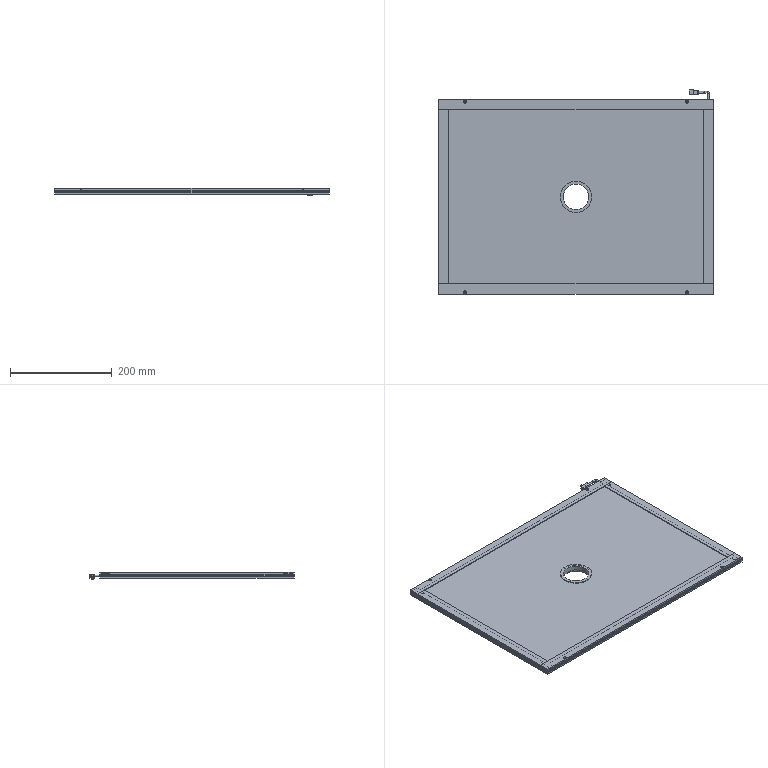Part | SolidWorks | 10 solids | 281 faces | box 540 x 401 x 14.65 mm | volume 2063206 mm3 | plane 200 | cylinder 75 | cone 4 | spline 2 | commonest cylinder face diameters 3.3 x16 6 x16 0.4 x8 2.076 x8 4.5 x8 3.8 x7